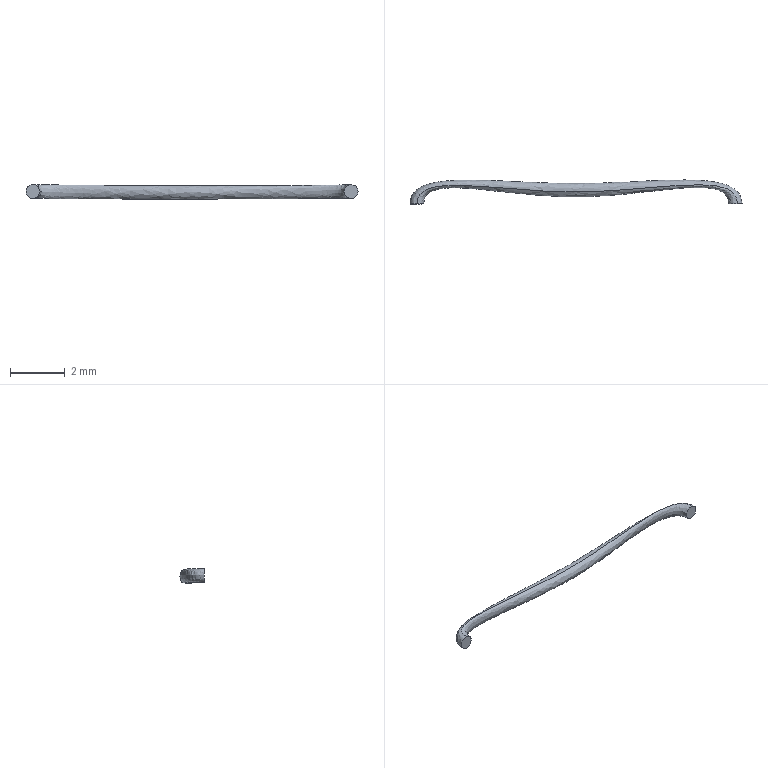Part | SolidWorks | features BaseBody 1 | 1 solid | 4 faces | box 12.097 x 0.8784 x 0.5345 mm | volume 1.852 mm3 | plane 2 | spline 2
STEP:
#1=CARTESIAN_POINT('',(336.128,424.458,120.514));
#2=VERTEX_POINT('',#1);
#3=CARTESIAN_POINT('',(336.12,424.458,120.014));
#4=VERTEX_POINT('',#3);
#5=CARTESIAN_POINT('',(336.128,424.458,120.514));
#6=CARTESIAN_POINT('',(336.095,424.458,120.515));
#7=CARTESIAN_POINT('',(336.027,424.458,120.502));
#8=CARTESIAN_POINT('',(335.946,424.458,120.448));
#9=CARTESIAN_POINT('',(335.89,424.458,120.369));
#10=CARTESIAN_POINT('',(335.869,424.458,120.275));
#11=CARTESIAN_POINT('',(335.882,424.458,120.187));
#12=CARTESIAN_POINT('',(335.929,424.458,120.094));
#13=CARTESIAN_POINT('',(335.997,424.458,120.041));
#14=CARTESIAN_POINT('',(336.06,424.458,120.022));
#15=CARTESIAN_POINT('',(336.08,424.458,120.018));
#16=CARTESIAN_POINT('',(336.1,424.458,120.015));
#17=CARTESIAN_POINT('',(336.113,424.458,120.014));
#18=CARTESIAN_POINT('',(336.12,424.458,120.014));
#19=B_SPLINE_CURVE_WITH_KNOTS('',3,(#5,#6,#7,#8,#9,#10,#11,#12,#13,#14,#15,#16,#17,#18),.UNSPECIFIED.,.F.,.F.,(4,1,1,1,1,1,1,1,1,1,1,4),(0.,0.125,0.25,0.375,0.5,0.6,0.7,0.9,0.925,0.95,0.975,1.),.UNSPECIFIED.);
#20=EDGE_CURVE('',#2,#4,#19,.T.);
#21=ORIENTED_EDGE('',*,*,#20,.T.);
#22=CARTESIAN_POINT('',(336.12,424.458,120.014));
#23=CARTESIAN_POINT('',(336.127,424.458,120.014));
#24=CARTESIAN_POINT('',(336.141,424.458,120.014));
#25=CARTESIAN_POINT('',(336.161,424.459,120.016));
#26=CARTESIAN_POINT('',(336.18,424.459,120.02));
#27=CARTESIAN_POINT('',(336.244,424.459,120.037));
#28=CARTESIAN_POINT('',(336.314,424.459,120.088));
#29=CARTESIAN_POINT('',(336.364,424.459,120.179));
#30=CARTESIAN_POINT('',(336.38,424.459,120.267));
#31=CARTESIAN_POINT('',(336.362,424.459,120.361));
#32=CARTESIAN_POINT('',(336.308,424.459,120.442));
#33=CARTESIAN_POINT('',(336.229,424.459,120.498));
#34=CARTESIAN_POINT('',(336.162,424.459,120.513));
#35=CARTESIAN_POINT('',(336.128,424.458,120.514));
#36=B_SPLINE_CURVE_WITH_KNOTS('',3,(#22,#23,#24,#25,#26,#27,#28,#29,#30,#31,#32,#33,#34,#35),.UNSPECIFIED.,.F.,.F.,(4,1,1,1,1,1,1,1,1,1,1,4),(0.,0.025,0.05,0.075,0.1,0.3,0.4,0.5,0.625,0.75,0.875,1.),.UNSPECIFIED.);
#37=EDGE_CURVE('',#4,#2,#36,.T.);
#38=ORIENTED_EDGE('',*,*,#37,.T.);
#39=EDGE_LOOP('',(#21,#38));
#40=FACE_OUTER_BOUND('',#39,.T.);
#41=CARTESIAN_POINT('',(336.124,424.458,120.264));
#42=DIRECTION('',(-0.0009599,1.,0.));
#43=DIRECTION('',(0.,0.,1.));
#44=AXIS2_PLACEMENT_3D('',#41,#42,#43);
#45=PLANE('',#44);
#46=ADVANCED_FACE('',(#40),#45,.F.);
#47=CARTESIAN_POINT('',(347.801,424.47,120.501));
#48=VERTEX_POINT('',#47);
#49=CARTESIAN_POINT('',(347.64,424.47,120.027));
#50=VERTEX_POINT('',#49);
#51=CARTESIAN_POINT('',(347.801,424.47,120.501));
#52=CARTESIAN_POINT('',(347.77,424.47,120.512));
#53=CARTESIAN_POINT('',(347.702,424.47,120.52));
#54=CARTESIAN_POINT('',(347.608,424.469,120.494));
#55=CARTESIAN_POINT('',(347.53,424.469,120.435));
#56=CARTESIAN_POINT('',(347.481,424.469,120.353));
#57=CARTESIAN_POINT('',(347.466,424.469,120.265));
#58=CARTESIAN_POINT('',(347.483,424.469,120.162));
#59=CARTESIAN_POINT('',(347.532,424.469,120.091));
#60=CARTESIAN_POINT('',(347.586,424.469,120.053));
#61=CARTESIAN_POINT('',(347.603,424.469,120.043));
#62=CARTESIAN_POINT('',(347.621,424.47,120.035));
#63=CARTESIAN_POINT('',(347.634,424.47,120.03));
#64=CARTESIAN_POINT('',(347.64,424.47,120.027));
#65=B_SPLINE_CURVE_WITH_KNOTS('',3,(#51,#52,#53,#54,#55,#56,#57,#58,#59,#60,#61,#62,#63,#64),.UNSPECIFIED.,.F.,.F.,(4,1,1,1,1,1,1,1,1,1,1,4),(0.,0.125,0.25,0.375,0.5,0.6,0.7,0.9,0.925,0.95,0.975,1.),.UNSPECIFIED.);
#66=EDGE_CURVE('',#48,#50,#65,.T.);
#67=ORIENTED_EDGE('',*,*,#66,.T.);
#68=CARTESIAN_POINT('',(347.64,424.47,120.027));
#69=CARTESIAN_POINT('',(347.647,424.47,120.025));
#70=CARTESIAN_POINT('',(347.66,424.47,120.021));
#71=CARTESIAN_POINT('',(347.68,424.47,120.017));
#72=CARTESIAN_POINT('',(347.699,424.47,120.015));
#73=CARTESIAN_POINT('',(347.765,424.47,120.012));
#74=CARTESIAN_POINT('',(347.848,424.47,120.038));
#75=CARTESIAN_POINT('',(347.923,424.47,120.11));
#76=CARTESIAN_POINT('',(347.965,424.47,120.188));
#77=CARTESIAN_POINT('',(347.977,424.47,120.283));
#78=CARTESIAN_POINT('',(347.95,424.47,120.377));
#79=CARTESIAN_POINT('',(347.892,424.47,120.455));
#80=CARTESIAN_POINT('',(347.833,424.47,120.49));
#81=CARTESIAN_POINT('',(347.801,424.47,120.501));
#82=B_SPLINE_CURVE_WITH_KNOTS('',3,(#68,#69,#70,#71,#72,#73,#74,#75,#76,#77,#78,#79,#80,#81),.UNSPECIFIED.,.F.,.F.,(4,1,1,1,1,1,1,1,1,1,1,4),(0.,0.025,0.05,0.075,0.1,0.3,0.4,0.5,0.625,0.75,0.875,1.),.UNSPECIFIED.);
#83=EDGE_CURVE('',#50,#48,#82,.T.);
#84=ORIENTED_EDGE('',*,*,#83,.T.);
#85=EDGE_LOOP('',(#67,#84));
#86=FACE_OUTER_BOUND('',#85,.T.);
#87=CARTESIAN_POINT('',(347.721,424.47,120.264));
#88=DIRECTION('',(-0.0009599,1.,0.));
#89=DIRECTION('',(0.,0.,1.));
#90=AXIS2_PLACEMENT_3D('',#87,#88,#89);
#91=PLANE('',#90);
#92=ADVANCED_FACE('',(#86),#91,.F.);
#93=CARTESIAN_POINT('',(336.128,424.458,120.514));
#94=CARTESIAN_POINT('',(336.127,425.678,120.514));
#95=CARTESIAN_POINT('',(341.881,424.101,120.435));
#96=CARTESIAN_POINT('',(347.8,425.706,120.501));
#97=CARTESIAN_POINT('',(347.801,424.47,120.501));
#98=B_SPLINE_CURVE_WITH_KNOTS('',3,(#93,#94,#95,#96,#97),.UNSPECIFIED.,.F.,.F.,(4,1,4),(0.,0.5,1.),.UNSPECIFIED.);
#99=EDGE_CURVE('',#2,#48,#98,.T.);
#100=ORIENTED_EDGE('',*,*,#99,.F.);
#101=ORIENTED_EDGE('',*,*,#37,.F.);
#102=CARTESIAN_POINT('',(347.64,424.47,120.027));
#103=CARTESIAN_POINT('',(347.639,425.694,120.027));
#104=CARTESIAN_POINT('',(341.965,424.365,119.959));
#105=CARTESIAN_POINT('',(336.119,425.7,120.014));
#106=CARTESIAN_POINT('',(336.12,424.458,120.014));
#107=B_SPLINE_CURVE_WITH_KNOTS('',3,(#102,#103,#104,#105,#106),.UNSPECIFIED.,.F.,.F.,(4,1,4),(0.,0.5,1.),.UNSPECIFIED.);
#108=EDGE_CURVE('',#50,#4,#107,.T.);
#109=ORIENTED_EDGE('',*,*,#108,.F.);
#110=ORIENTED_EDGE('',*,*,#66,.F.);
#111=EDGE_LOOP('',(#100,#101,#109,#110));
#112=FACE_OUTER_BOUND('',#111,.T.);
#113=CARTESIAN_POINT('',(347.807,424.347,120.495));
#114=CARTESIAN_POINT('',(348.,425.761,120.497));
#115=CARTESIAN_POINT('',(341.87,424.074,120.444));
#116=CARTESIAN_POINT('',(335.914,425.737,120.516));
#117=CARTESIAN_POINT('',(336.123,424.326,120.514));
#118=CARTESIAN_POINT('',(347.802,424.347,120.497));
#119=CARTESIAN_POINT('',(347.995,425.76,120.499));
#120=CARTESIAN_POINT('',(341.87,424.065,120.44));
#121=CARTESIAN_POINT('',(335.92,425.736,120.517));
#122=CARTESIAN_POINT('',(336.128,424.326,120.514));
#123=CARTESIAN_POINT('',(347.766,424.348,120.511));
#124=CARTESIAN_POINT('',(347.958,425.75,120.514));
#125=CARTESIAN_POINT('',(341.868,424.,120.414));
#126=CARTESIAN_POINT('',(335.96,425.725,120.518));
#127=CARTESIAN_POINT('',(336.167,424.327,120.514));
#128=CARTESIAN_POINT('',(347.693,424.35,120.52));
#129=CARTESIAN_POINT('',(347.883,425.73,120.525));
#130=CARTESIAN_POINT('',(341.869,423.889,120.347));
#131=CARTESIAN_POINT('',(336.034,425.707,120.504));
#132=CARTESIAN_POINT('',(336.239,424.329,120.498));
#133=CARTESIAN_POINT('',(347.599,424.353,120.493));
#134=CARTESIAN_POINT('',(347.786,425.704,120.502));
#135=CARTESIAN_POINT('',(341.877,423.788,120.237));
#136=CARTESIAN_POINT('',(336.116,425.684,120.449));
#137=CARTESIAN_POINT('',(336.318,424.332,120.442));
#138=CARTESIAN_POINT('',(347.521,424.355,120.435));
#139=CARTESIAN_POINT('',(347.705,425.684,120.445));
#140=CARTESIAN_POINT('',(341.89,423.743,120.121));
#141=CARTESIAN_POINT('',(336.171,425.669,120.369));
#142=CARTESIAN_POINT('',(336.372,424.334,120.36));
#143=CARTESIAN_POINT('',(347.473,424.356,120.352));
#144=CARTESIAN_POINT('',(347.654,425.673,120.363));
#145=CARTESIAN_POINT('',(341.907,423.763,120.018));
#146=CARTESIAN_POINT('',(336.189,425.664,120.275));
#147=CARTESIAN_POINT('',(336.39,424.334,120.266));
#148=CARTESIAN_POINT('',(347.458,424.355,120.265));
#149=CARTESIAN_POINT('',(347.639,425.673,120.275));
#150=CARTESIAN_POINT('',(341.923,423.836,119.944));
#151=CARTESIAN_POINT('',(336.172,425.67,120.187));
#152=CARTESIAN_POINT('',(336.374,424.333,120.179));
#153=CARTESIAN_POINT('',(347.474,424.354,120.162));
#154=CARTESIAN_POINT('',(347.655,425.683,120.171));
#155=CARTESIAN_POINT('',(341.941,423.965,119.892));
#156=CARTESIAN_POINT('',(336.12,425.686,120.095));
#157=CARTESIAN_POINT('',(336.324,424.331,120.088));
#158=CARTESIAN_POINT('',(347.524,424.352,120.091));
#159=CARTESIAN_POINT('',(347.705,425.701,120.097));
#160=CARTESIAN_POINT('',(341.952,424.106,119.892));
#161=CARTESIAN_POINT('',(336.047,425.709,120.042));
#162=CARTESIAN_POINT('',(336.254,424.329,120.037));
#163=CARTESIAN_POINT('',(347.577,424.351,120.053));
#164=CARTESIAN_POINT('',(347.76,425.719,120.058));
#165=CARTESIAN_POINT('',(341.957,424.219,119.92));
#166=CARTESIAN_POINT('',(335.981,425.728,120.024));
#167=CARTESIAN_POINT('',(336.191,424.326,120.02));
#168=CARTESIAN_POINT('',(347.595,424.35,120.043));
#169=CARTESIAN_POINT('',(347.778,425.725,120.047));
#170=CARTESIAN_POINT('',(341.958,424.253,119.931));
#171=CARTESIAN_POINT('',(335.961,425.734,120.019));
#172=CARTESIAN_POINT('',(336.171,424.326,120.016));
#173=CARTESIAN_POINT('',(347.613,424.349,120.034));
#174=CARTESIAN_POINT('',(347.797,425.731,120.037));
#175=CARTESIAN_POINT('',(341.959,424.287,119.943));
#176=CARTESIAN_POINT('',(335.94,425.74,120.017));
#177=CARTESIAN_POINT('',(336.151,424.325,120.014));
#178=CARTESIAN_POINT('',(347.63,424.349,120.028));
#179=CARTESIAN_POINT('',(347.815,425.736,120.03));
#180=CARTESIAN_POINT('',(341.96,424.319,119.956));
#181=CARTESIAN_POINT('',(335.921,425.746,120.016));
#182=CARTESIAN_POINT('',(336.132,424.324,120.014));
#183=CARTESIAN_POINT('',(347.642,424.349,120.024));
#184=CARTESIAN_POINT('',(347.827,425.74,120.026));
#185=CARTESIAN_POINT('',(341.96,424.338,119.965));
#186=CARTESIAN_POINT('',(335.908,425.75,120.016));
#187=CARTESIAN_POINT('',(336.12,424.324,120.014));
#188=CARTESIAN_POINT('',(347.647,424.348,120.023));
#189=CARTESIAN_POINT('',(347.832,425.741,120.024));
#190=CARTESIAN_POINT('',(341.96,424.346,119.969));
#191=CARTESIAN_POINT('',(335.903,425.751,120.016));
#192=CARTESIAN_POINT('',(336.115,424.324,120.015));
#193=B_SPLINE_SURFACE_WITH_KNOTS('',3,3,((#113,#114,#115,#116,#117),(#118,#119,#120,#121,#122),(#123,#124,#125,#126,#127),(#128,#129,#130,#131,#132),(#133,#134,#135,#136,#137),(#138,#139,#140,#141,#142),(#143,#144,#145,#146,#147),(#148,#149,#150,#151,#152),(#153,#154,#155,#156,#157),(#158,#159,#160,#161,#162),(#163,#164,#165,#166,#167),(#168,#169,#170,#171,#172),(#173,#174,#175,#176,#177),(#178,#179,#180,#181,#182),(#183,#184,#185,#186,#187),(#188,#189,#190,#191,#192)),.UNSPECIFIED.,.F.,.F.,.F.,(4,1,1,1,1,1,1,1,1,1,1,1,1,4),(4,1,4),(0.4905,0.5,0.5625,0.625,0.6875,0.75,0.8,0.85,0.95,0.9625,0.975,0.9875,1.,1.01),(-0.01566,0.5,1.017),.UNSPECIFIED.);
#194=ADVANCED_FACE('',(#112),#193,.F.);
#195=ORIENTED_EDGE('',*,*,#83,.F.);
#196=ORIENTED_EDGE('',*,*,#108,.T.);
#197=ORIENTED_EDGE('',*,*,#20,.F.);
#198=ORIENTED_EDGE('',*,*,#99,.T.);
#199=EDGE_LOOP('',(#195,#196,#197,#198));
#200=FACE_OUTER_BOUND('',#199,.T.);
#201=CARTESIAN_POINT('',(347.617,424.349,120.033));
#202=CARTESIAN_POINT('',(347.802,425.732,120.036));
#203=CARTESIAN_POINT('',(341.959,424.295,119.946));
#204=CARTESIAN_POINT('',(335.935,425.742,120.017));
#205=CARTESIAN_POINT('',(336.146,424.325,120.014));
#206=CARTESIAN_POINT('',(347.622,424.349,120.031));
#207=CARTESIAN_POINT('',(347.807,425.734,120.033));
#208=CARTESIAN_POINT('',(341.959,424.304,119.95));
#209=CARTESIAN_POINT('',(335.93,425.743,120.016));
#210=CARTESIAN_POINT('',(336.141,424.325,120.014));
#211=CARTESIAN_POINT('',(347.633,424.349,120.027));
#212=CARTESIAN_POINT('',(347.818,425.737,120.029));
#213=CARTESIAN_POINT('',(341.96,424.324,119.958));
#214=CARTESIAN_POINT('',(335.917,425.747,120.016));
#215=CARTESIAN_POINT('',(336.129,424.324,120.014));
#216=CARTESIAN_POINT('',(347.652,424.348,120.021));
#217=CARTESIAN_POINT('',(347.837,425.743,120.023));
#218=CARTESIAN_POINT('',(341.96,424.354,119.972));
#219=CARTESIAN_POINT('',(335.898,425.753,120.016));
#220=CARTESIAN_POINT('',(336.11,424.323,120.015));
#221=CARTESIAN_POINT('',(347.671,424.348,120.017));
#222=CARTESIAN_POINT('',(347.857,425.749,120.018));
#223=CARTESIAN_POINT('',(341.96,424.386,119.989));
#224=CARTESIAN_POINT('',(335.877,425.759,120.019));
#225=CARTESIAN_POINT('',(336.09,424.323,120.018));
#226=CARTESIAN_POINT('',(347.691,424.347,120.015));
#227=CARTESIAN_POINT('',(347.878,425.755,120.015));
#228=CARTESIAN_POINT('',(341.96,424.415,120.007));
#229=CARTESIAN_POINT('',(335.857,425.765,120.023));
#230=CARTESIAN_POINT('',(336.071,424.322,120.022));
#231=CARTESIAN_POINT('',(347.757,424.345,120.012));
#232=CARTESIAN_POINT('',(347.946,425.774,120.01));
#233=CARTESIAN_POINT('',(341.958,424.508,120.07));
#234=CARTESIAN_POINT('',(335.792,425.783,120.041));
#235=CARTESIAN_POINT('',(336.008,424.32,120.042));
#236=CARTESIAN_POINT('',(347.839,424.343,120.038));
#237=CARTESIAN_POINT('',(348.031,425.798,120.034));
#238=CARTESIAN_POINT('',(341.951,424.592,120.169));
#239=CARTESIAN_POINT('',(335.721,425.803,120.092));
#240=CARTESIAN_POINT('',(335.94,424.318,120.094));
#241=CARTESIAN_POINT('',(347.914,424.341,120.11));
#242=CARTESIAN_POINT('',(348.109,425.816,120.104));
#243=CARTESIAN_POINT('',(341.935,424.62,120.291));
#244=CARTESIAN_POINT('',(335.673,425.815,120.184));
#245=CARTESIAN_POINT('',(335.893,424.316,120.187));
#246=CARTESIAN_POINT('',(347.956,424.34,120.189));
#247=CARTESIAN_POINT('',(348.153,425.824,120.182));
#248=CARTESIAN_POINT('',(341.92,424.596,120.386));
#249=CARTESIAN_POINT('',(335.66,425.817,120.271));
#250=CARTESIAN_POINT('',(335.88,424.316,120.275));
#251=CARTESIAN_POINT('',(347.968,424.341,120.284));
#252=CARTESIAN_POINT('',(348.165,425.82,120.278));
#253=CARTESIAN_POINT('',(341.902,424.515,120.461));
#254=CARTESIAN_POINT('',(335.683,425.808,120.365));
#255=CARTESIAN_POINT('',(335.901,424.317,120.369));
#256=CARTESIAN_POINT('',(347.941,424.342,120.377));
#257=CARTESIAN_POINT('',(348.139,425.806,120.373));
#258=CARTESIAN_POINT('',(341.886,424.383,120.498));
#259=CARTESIAN_POINT('',(335.741,425.787,120.446));
#260=CARTESIAN_POINT('',(335.957,424.32,120.448));
#261=CARTESIAN_POINT('',(347.883,424.345,120.455));
#262=CARTESIAN_POINT('',(348.079,425.784,120.454));
#263=CARTESIAN_POINT('',(341.874,424.223,120.492));
#264=CARTESIAN_POINT('',(335.826,425.761,120.502));
#265=CARTESIAN_POINT('',(336.038,424.323,120.502));
#266=CARTESIAN_POINT('',(347.82,424.347,120.493));
#267=CARTESIAN_POINT('',(348.014,425.765,120.494));
#268=CARTESIAN_POINT('',(341.87,424.095,120.455));
#269=CARTESIAN_POINT('',(335.901,425.741,120.518));
#270=CARTESIAN_POINT('',(336.11,424.325,120.515));
#271=CARTESIAN_POINT('',(347.783,424.348,120.504));
#272=CARTESIAN_POINT('',(347.975,425.755,120.506));
#273=CARTESIAN_POINT('',(341.869,424.031,120.426));
#274=CARTESIAN_POINT('',(335.941,425.73,120.517));
#275=CARTESIAN_POINT('',(336.149,424.326,120.514));
#276=CARTESIAN_POINT('',(347.778,424.348,120.505));
#277=CARTESIAN_POINT('',(347.97,425.753,120.508));
#278=CARTESIAN_POINT('',(341.869,424.023,120.422));
#279=CARTESIAN_POINT('',(335.946,425.729,120.516));
#280=CARTESIAN_POINT('',(336.154,424.327,120.513));
#281=B_SPLINE_SURFACE_WITH_KNOTS('',3,3,((#201,#202,#203,#204,#205),(#206,#207,#208,#209,#210),(#211,#212,#213,#214,#215),(#216,#217,#218,#219,#220),(#221,#222,#223,#224,#225),(#226,#227,#228,#229,#230),(#231,#232,#233,#234,#235),(#236,#237,#238,#239,#240),(#241,#242,#243,#244,#245),(#246,#247,#248,#249,#250),(#251,#252,#253,#254,#255),(#256,#257,#258,#259,#260),(#261,#262,#263,#264,#265),(#266,#267,#268,#269,#270),(#271,#272,#273,#274,#275),(#276,#277,#278,#279,#280)),.UNSPECIFIED.,.F.,.F.,.F.,(4,1,1,1,1,1,1,1,1,1,1,1,1,4),(4,1,4),(-0.009538,0.,0.0125,0.025,0.0375,0.05,0.15,0.2,0.25,0.3125,0.375,0.4375,0.5,0.5095),(-0.01566,0.5,1.017),.UNSPECIFIED.);
#282=ADVANCED_FACE('',(#200),#281,.F.);
#283=CLOSED_SHELL('',(#46,#92,#194,#282));
#284=MANIFOLD_SOLID_BREP('',#283);
#285=CARTESIAN_POINT('',(0.,0.,0.));
#286=DIRECTION('',(0.,0.,1.));
#287=DIRECTION('',(1.,0.,0.));
#288=AXIS2_PLACEMENT_3D('',#285,#286,#287);
#289=(LENGTH_UNIT()NAMED_UNIT(*)SI_UNIT(.MILLI.,.METRE.));
#290=UNCERTAINTY_MEASURE_WITH_UNIT(LENGTH_MEASURE(0.00001),#289,'','');
#291=(NAMED_UNIT(*)PLANE_ANGLE_UNIT()SI_UNIT($,.RADIAN.));
#292=(NAMED_UNIT(*)SI_UNIT($,.STERADIAN.)SOLID_ANGLE_UNIT());
#293=(GEOMETRIC_REPRESENTATION_CONTEXT(3)GLOBAL_UNCERTAINTY_ASSIGNED_CONTEXT((#290))GLOBAL_UNIT_ASSIGNED_CONTEXT((#289,#291,#292))REPRESENTATION_CONTEXT('',''));
#294=ADVANCED_BREP_SHAPE_REPRESENTATION('',(#284,#288),#293);